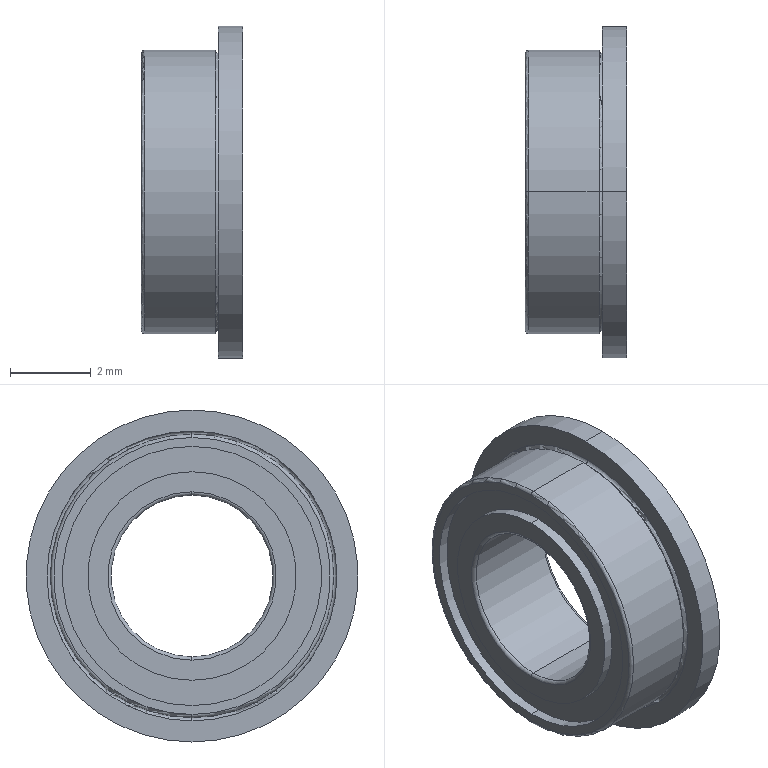Part | SolidWorks | features RefAxis 3, 3DProfileFeature 1, Revolution 1 | 1 solid | 31 faces | box 2.5 x 8.2 x 8.2 mm | volume 67.212 mm3 | cylinder 14 | torus 10 | plane 7 | commonest cylinder face diameters 5.15 x4 6.4 x4 4 x2 7 x2 8.2 x2
STEP:
#1=CARTESIAN_POINT('',(1.82,0.,3.5));
#2=VERTEX_POINT('',#1);
#3=CARTESIAN_POINT('',(1.9,0.,3.42));
#4=VERTEX_POINT('',#3);
#5=CARTESIAN_POINT('',(1.9,0.,3.5));
#6=DIRECTION('',(0.,-1.,0.));
#7=DIRECTION('',(0.,0.,-1.));
#8=AXIS2_PLACEMENT_3D('',#5,#6,#7);
#9=CIRCLE('',#8,0.08);
#10=EDGE_CURVE('',#2,#4,#9,.T.);
#11=ORIENTED_EDGE('',*,*,#10,.T.);
#12=CARTESIAN_POINT('',(1.9,0.,-3.42));
#13=VERTEX_POINT('',#12);
#14=CARTESIAN_POINT('',(1.9,0.,0.));
#15=DIRECTION('',(-1.,0.,0.));
#16=DIRECTION('',(0.,0.,1.));
#17=AXIS2_PLACEMENT_3D('',#14,#15,#16);
#18=CIRCLE('',#17,3.42);
#19=EDGE_CURVE('',#4,#13,#18,.T.);
#20=ORIENTED_EDGE('',*,*,#19,.T.);
#21=CARTESIAN_POINT('',(1.82,0.,-3.5));
#22=VERTEX_POINT('',#21);
#23=CARTESIAN_POINT('',(1.9,0.,-3.5));
#24=DIRECTION('',(0.,1.,0.));
#25=DIRECTION('',(0.,0.,1.));
#26=AXIS2_PLACEMENT_3D('',#23,#24,#25);
#27=CIRCLE('',#26,0.08);
#28=EDGE_CURVE('',#22,#13,#27,.T.);
#29=ORIENTED_EDGE('',*,*,#28,.F.);
#30=CARTESIAN_POINT('',(1.82,0.,0.));
#31=DIRECTION('',(-1.,0.,0.));
#32=DIRECTION('',(0.,0.,1.));
#33=AXIS2_PLACEMENT_3D('',#30,#31,#32);
#34=CIRCLE('',#33,3.5);
#35=EDGE_CURVE('',#2,#22,#34,.T.);
#36=ORIENTED_EDGE('',*,*,#35,.F.);
#37=EDGE_LOOP('',(#11,#20,#29,#36));
#38=FACE_OUTER_BOUND('',#37,.T.);
#39=CARTESIAN_POINT('',(1.9,0.,0.));
#40=DIRECTION('',(-1.,0.,0.));
#41=DIRECTION('',(0.,0.,1.));
#42=AXIS2_PLACEMENT_3D('',#39,#40,#41);
#43=TOROIDAL_SURFACE('',#42,3.5,0.08);
#44=ADVANCED_FACE('',(#38),#43,.F.);
#45=ORIENTED_EDGE('',*,*,#28,.T.);
#46=CARTESIAN_POINT('',(1.9,0.,0.));
#47=DIRECTION('',(-1.,0.,0.));
#48=DIRECTION('',(0.,0.,1.));
#49=AXIS2_PLACEMENT_3D('',#46,#47,#48);
#50=CIRCLE('',#49,3.42);
#51=EDGE_CURVE('',#13,#4,#50,.T.);
#52=ORIENTED_EDGE('',*,*,#51,.T.);
#53=ORIENTED_EDGE('',*,*,#10,.F.);
#54=CARTESIAN_POINT('',(1.82,0.,0.));
#55=DIRECTION('',(-1.,0.,0.));
#56=DIRECTION('',(0.,0.,1.));
#57=AXIS2_PLACEMENT_3D('',#54,#55,#56);
#58=CIRCLE('',#57,3.5);
#59=EDGE_CURVE('',#22,#2,#58,.T.);
#60=ORIENTED_EDGE('',*,*,#59,.F.);
#61=EDGE_LOOP('',(#45,#52,#53,#60));
#62=FACE_OUTER_BOUND('',#61,.T.);
#63=CARTESIAN_POINT('',(1.9,0.,0.));
#64=DIRECTION('',(-1.,0.,0.));
#65=DIRECTION('',(0.,0.,1.));
#66=AXIS2_PLACEMENT_3D('',#63,#64,#65);
#67=TOROIDAL_SURFACE('',#66,3.5,0.08);
#68=ADVANCED_FACE('',(#62),#67,.F.);
#69=ORIENTED_EDGE('',*,*,#35,.T.);
#70=CARTESIAN_POINT('',(0.08,0.,-3.5));
#71=VERTEX_POINT('',#70);
#72=CARTESIAN_POINT('',(7.,0.,-3.5));
#73=DIRECTION('',(-1.,0.,0.));
#74=VECTOR('',#73,1000.);
#75=LINE('',#72,#74);
#76=EDGE_CURVE('',#22,#71,#75,.T.);
#77=ORIENTED_EDGE('',*,*,#76,.T.);
#78=CARTESIAN_POINT('',(0.08,0.,3.5));
#79=VERTEX_POINT('',#78);
#80=CARTESIAN_POINT('',(0.08,0.,0.));
#81=DIRECTION('',(-1.,0.,0.));
#82=DIRECTION('',(0.,0.,1.));
#83=AXIS2_PLACEMENT_3D('',#80,#81,#82);
#84=CIRCLE('',#83,3.5);
#85=EDGE_CURVE('',#79,#71,#84,.T.);
#86=ORIENTED_EDGE('',*,*,#85,.F.);
#87=CARTESIAN_POINT('',(7.,0.,3.5));
#88=DIRECTION('',(-1.,0.,0.));
#89=VECTOR('',#88,1000.);
#90=LINE('',#87,#89);
#91=EDGE_CURVE('',#2,#79,#90,.T.);
#92=ORIENTED_EDGE('',*,*,#91,.F.);
#93=EDGE_LOOP('',(#69,#77,#86,#92));
#94=FACE_OUTER_BOUND('',#93,.T.);
#95=CARTESIAN_POINT('',(7.,0.,0.));
#96=DIRECTION('',(-1.,0.,0.));
#97=DIRECTION('',(0.,0.,1.));
#98=AXIS2_PLACEMENT_3D('',#95,#96,#97);
#99=CYLINDRICAL_SURFACE('',#98,3.5);
#100=ADVANCED_FACE('',(#94),#99,.T.);
#101=ORIENTED_EDGE('',*,*,#51,.F.);
#102=CARTESIAN_POINT('',(1.9,0.,-3.58));
#103=VERTEX_POINT('',#102);
#104=CARTESIAN_POINT('',(1.9,0.,-3.5));
#105=DIRECTION('',(0.,1.,0.));
#106=DIRECTION('',(0.,0.,1.));
#107=AXIS2_PLACEMENT_3D('',#104,#105,#106);
#108=CIRCLE('',#107,0.08);
#109=EDGE_CURVE('',#13,#103,#108,.T.);
#110=ORIENTED_EDGE('',*,*,#109,.T.);
#111=CARTESIAN_POINT('',(1.9,0.,3.58));
#112=VERTEX_POINT('',#111);
#113=CARTESIAN_POINT('',(1.9,0.,0.));
#114=DIRECTION('',(-1.,0.,0.));
#115=DIRECTION('',(0.,0.,1.));
#116=AXIS2_PLACEMENT_3D('',#113,#114,#115);
#117=CIRCLE('',#116,3.58);
#118=EDGE_CURVE('',#103,#112,#117,.T.);
#119=ORIENTED_EDGE('',*,*,#118,.T.);
#120=CARTESIAN_POINT('',(1.9,0.,3.5));
#121=DIRECTION('',(0.,-1.,0.));
#122=DIRECTION('',(0.,0.,-1.));
#123=AXIS2_PLACEMENT_3D('',#120,#121,#122);
#124=CIRCLE('',#123,0.08);
#125=EDGE_CURVE('',#4,#112,#124,.T.);
#126=ORIENTED_EDGE('',*,*,#125,.F.);
#127=EDGE_LOOP('',(#101,#110,#119,#126));
#128=FACE_OUTER_BOUND('',#127,.T.);
#129=CARTESIAN_POINT('',(1.9,0.,0.));
#130=DIRECTION('',(-1.,0.,0.));
#131=DIRECTION('',(0.,0.,1.));
#132=AXIS2_PLACEMENT_3D('',#129,#130,#131);
#133=TOROIDAL_SURFACE('',#132,3.5,0.08);
#134=ADVANCED_FACE('',(#128),#133,.F.);
#135=CARTESIAN_POINT('',(2.5,0.,4.1));
#136=VERTEX_POINT('',#135);
#137=CARTESIAN_POINT('',(2.5,0.,-4.1));
#138=VERTEX_POINT('',#137);
#139=CARTESIAN_POINT('',(2.5,0.,0.));
#140=DIRECTION('',(-1.,0.,0.));
#141=DIRECTION('',(0.,0.,1.));
#142=AXIS2_PLACEMENT_3D('',#139,#140,#141);
#143=CIRCLE('',#142,4.1);
#144=EDGE_CURVE('',#136,#138,#143,.T.);
#145=ORIENTED_EDGE('',*,*,#144,.T.);
#146=CARTESIAN_POINT('',(1.9,0.,-4.1));
#147=VERTEX_POINT('',#146);
#148=CARTESIAN_POINT('',(7.,0.,-4.1));
#149=DIRECTION('',(-1.,0.,0.));
#150=VECTOR('',#149,1000.);
#151=LINE('',#148,#150);
#152=EDGE_CURVE('',#138,#147,#151,.T.);
#153=ORIENTED_EDGE('',*,*,#152,.T.);
#154=CARTESIAN_POINT('',(1.9,0.,4.1));
#155=VERTEX_POINT('',#154);
#156=CARTESIAN_POINT('',(1.9,0.,0.));
#157=DIRECTION('',(-1.,0.,0.));
#158=DIRECTION('',(0.,0.,1.));
#159=AXIS2_PLACEMENT_3D('',#156,#157,#158);
#160=CIRCLE('',#159,4.1);
#161=EDGE_CURVE('',#155,#147,#160,.T.);
#162=ORIENTED_EDGE('',*,*,#161,.F.);
#163=CARTESIAN_POINT('',(7.,0.,4.1));
#164=DIRECTION('',(-1.,0.,0.));
#165=VECTOR('',#164,1000.);
#166=LINE('',#163,#165);
#167=EDGE_CURVE('',#136,#155,#166,.T.);
#168=ORIENTED_EDGE('',*,*,#167,.F.);
#169=EDGE_LOOP('',(#145,#153,#162,#168));
#170=FACE_OUTER_BOUND('',#169,.T.);
#171=CARTESIAN_POINT('',(7.,0.,0.));
#172=DIRECTION('',(-1.,0.,0.));
#173=DIRECTION('',(0.,0.,1.));
#174=AXIS2_PLACEMENT_3D('',#171,#172,#173);
#175=CYLINDRICAL_SURFACE('',#174,4.1);
#176=ADVANCED_FACE('',(#170),#175,.T.);
#177=CARTESIAN_POINT('',(2.5,0.,-3.2));
#178=VERTEX_POINT('',#177);
#179=CARTESIAN_POINT('',(2.5,0.,3.2));
#180=VERTEX_POINT('',#179);
#181=CARTESIAN_POINT('',(2.5,0.,0.));
#182=DIRECTION('',(-1.,0.,0.));
#183=DIRECTION('',(0.,0.,1.));
#184=AXIS2_PLACEMENT_3D('',#181,#182,#183);
#185=CIRCLE('',#184,3.2);
#186=EDGE_CURVE('',#178,#180,#185,.T.);
#187=ORIENTED_EDGE('',*,*,#186,.F.);
#188=CARTESIAN_POINT('',(2.245,0.,-3.2));
#189=VERTEX_POINT('',#188);
#190=CARTESIAN_POINT('',(7.,0.,-3.2));
#191=DIRECTION('',(-1.,0.,0.));
#192=VECTOR('',#191,1000.);
#193=LINE('',#190,#192);
#194=EDGE_CURVE('',#178,#189,#193,.T.);
#195=ORIENTED_EDGE('',*,*,#194,.T.);
#196=CARTESIAN_POINT('',(2.245,0.,3.2));
#197=VERTEX_POINT('',#196);
#198=CARTESIAN_POINT('',(2.245,0.,0.));
#199=DIRECTION('',(-1.,0.,0.));
#200=DIRECTION('',(0.,0.,1.));
#201=AXIS2_PLACEMENT_3D('',#198,#199,#200);
#202=CIRCLE('',#201,3.2);
#203=EDGE_CURVE('',#189,#197,#202,.T.);
#204=ORIENTED_EDGE('',*,*,#203,.T.);
#205=CARTESIAN_POINT('',(7.,0.,3.2));
#206=DIRECTION('',(-1.,0.,0.));
#207=VECTOR('',#206,1000.);
#208=LINE('',#205,#207);
#209=EDGE_CURVE('',#180,#197,#208,.T.);
#210=ORIENTED_EDGE('',*,*,#209,.F.);
#211=EDGE_LOOP('',(#187,#195,#204,#210));
#212=FACE_OUTER_BOUND('',#211,.T.);
#213=CARTESIAN_POINT('',(7.,0.,0.));
#214=DIRECTION('',(-1.,0.,0.));
#215=DIRECTION('',(0.,0.,1.));
#216=AXIS2_PLACEMENT_3D('',#213,#214,#215);
#217=CYLINDRICAL_SURFACE('',#216,3.2);
#218=ADVANCED_FACE('',(#212),#217,.F.);
#219=CARTESIAN_POINT('',(2.5,0.,2.575));
#220=VERTEX_POINT('',#219);
#221=CARTESIAN_POINT('',(2.5,0.,-2.575));
#222=VERTEX_POINT('',#221);
#223=CARTESIAN_POINT('',(2.5,0.,0.));
#224=DIRECTION('',(-1.,0.,0.));
#225=DIRECTION('',(0.,0.,1.));
#226=AXIS2_PLACEMENT_3D('',#223,#224,#225);
#227=CIRCLE('',#226,2.575);
#228=EDGE_CURVE('',#220,#222,#227,.T.);
#229=ORIENTED_EDGE('',*,*,#228,.T.);
#230=CARTESIAN_POINT('',(2.245,0.,-2.575));
#231=VERTEX_POINT('',#230);
#232=CARTESIAN_POINT('',(7.,0.,-2.575));
#233=DIRECTION('',(-1.,0.,0.));
#234=VECTOR('',#233,1000.);
#235=LINE('',#232,#234);
#236=EDGE_CURVE('',#222,#231,#235,.T.);
#237=ORIENTED_EDGE('',*,*,#236,.T.);
#238=CARTESIAN_POINT('',(2.245,0.,2.575));
#239=VERTEX_POINT('',#238);
#240=CARTESIAN_POINT('',(2.245,0.,0.));
#241=DIRECTION('',(-1.,0.,0.));
#242=DIRECTION('',(0.,0.,1.));
#243=AXIS2_PLACEMENT_3D('',#240,#241,#242);
#244=CIRCLE('',#243,2.575);
#245=EDGE_CURVE('',#239,#231,#244,.T.);
#246=ORIENTED_EDGE('',*,*,#245,.F.);
#247=CARTESIAN_POINT('',(7.,0.,2.575));
#248=DIRECTION('',(-1.,0.,0.));
#249=VECTOR('',#248,1000.);
#250=LINE('',#247,#249);
#251=EDGE_CURVE('',#220,#239,#250,.T.);
#252=ORIENTED_EDGE('',*,*,#251,.F.);
#253=EDGE_LOOP('',(#229,#237,#246,#252));
#254=FACE_OUTER_BOUND('',#253,.T.);
#255=CARTESIAN_POINT('',(7.,0.,0.));
#256=DIRECTION('',(-1.,0.,0.));
#257=DIRECTION('',(0.,0.,1.));
#258=AXIS2_PLACEMENT_3D('',#255,#256,#257);
#259=CYLINDRICAL_SURFACE('',#258,2.575);
#260=ADVANCED_FACE('',(#254),#259,.T.);
#261=CARTESIAN_POINT('',(2.42,0.,2.));
#262=VERTEX_POINT('',#261);
#263=CARTESIAN_POINT('',(2.42,0.,-2.));
#264=VERTEX_POINT('',#263);
#265=CARTESIAN_POINT('',(2.42,0.,0.));
#266=DIRECTION('',(-1.,0.,0.));
#267=DIRECTION('',(0.,0.,1.));
#268=AXIS2_PLACEMENT_3D('',#265,#266,#267);
#269=CIRCLE('',#268,2.);
#270=EDGE_CURVE('',#262,#264,#269,.T.);
#271=ORIENTED_EDGE('',*,*,#270,.T.);
#272=CARTESIAN_POINT('',(2.5,0.,-2.08));
#273=VERTEX_POINT('',#272);
#274=CARTESIAN_POINT('',(2.42,0.,-2.08));
#275=DIRECTION('',(0.,1.,0.));
#276=DIRECTION('',(0.,0.,1.));
#277=AXIS2_PLACEMENT_3D('',#274,#275,#276);
#278=CIRCLE('',#277,0.08);
#279=EDGE_CURVE('',#264,#273,#278,.T.);
#280=ORIENTED_EDGE('',*,*,#279,.T.);
#281=CARTESIAN_POINT('',(2.5,0.,2.08));
#282=VERTEX_POINT('',#281);
#283=CARTESIAN_POINT('',(2.5,0.,0.));
#284=DIRECTION('',(-1.,0.,0.));
#285=DIRECTION('',(0.,0.,1.));
#286=AXIS2_PLACEMENT_3D('',#283,#284,#285);
#287=CIRCLE('',#286,2.08);
#288=EDGE_CURVE('',#282,#273,#287,.T.);
#289=ORIENTED_EDGE('',*,*,#288,.F.);
#290=CARTESIAN_POINT('',(2.42,0.,2.08));
#291=DIRECTION('',(0.,-1.,0.));
#292=DIRECTION('',(0.,0.,-1.));
#293=AXIS2_PLACEMENT_3D('',#290,#291,#292);
#294=CIRCLE('',#293,0.08);
#295=EDGE_CURVE('',#262,#282,#294,.T.);
#296=ORIENTED_EDGE('',*,*,#295,.F.);
#297=EDGE_LOOP('',(#271,#280,#289,#296));
#298=FACE_OUTER_BOUND('',#297,.T.);
#299=CARTESIAN_POINT('',(2.42,0.,0.));
#300=DIRECTION('',(-1.,0.,0.));
#301=DIRECTION('',(0.,0.,1.));
#302=AXIS2_PLACEMENT_3D('',#299,#300,#301);
#303=TOROIDAL_SURFACE('',#302,2.08,0.08);
#304=ADVANCED_FACE('',(#298),#303,.T.);
#305=CARTESIAN_POINT('',(2.42,0.,0.));
#306=DIRECTION('',(-1.,0.,0.));
#307=DIRECTION('',(0.,0.,1.));
#308=AXIS2_PLACEMENT_3D('',#305,#306,#307);
#309=CIRCLE('',#308,2.);
#310=EDGE_CURVE('',#264,#262,#309,.T.);
#311=ORIENTED_EDGE('',*,*,#310,.F.);
#312=CARTESIAN_POINT('',(0.08,0.,-2.));
#313=VERTEX_POINT('',#312);
#314=CARTESIAN_POINT('',(7.,0.,-2.));
#315=DIRECTION('',(-1.,0.,0.));
#316=VECTOR('',#315,1000.);
#317=LINE('',#314,#316);
#318=EDGE_CURVE('',#264,#313,#317,.T.);
#319=ORIENTED_EDGE('',*,*,#318,.T.);
#320=CARTESIAN_POINT('',(0.08,0.,2.));
#321=VERTEX_POINT('',#320);
#322=CARTESIAN_POINT('',(0.08,0.,0.));
#323=DIRECTION('',(-1.,0.,0.));
#324=DIRECTION('',(0.,0.,1.));
#325=AXIS2_PLACEMENT_3D('',#322,#323,#324);
#326=CIRCLE('',#325,2.);
#327=EDGE_CURVE('',#313,#321,#326,.T.);
#328=ORIENTED_EDGE('',*,*,#327,.T.);
#329=CARTESIAN_POINT('',(7.,0.,2.));
#330=DIRECTION('',(-1.,0.,0.));
#331=VECTOR('',#330,1000.);
#332=LINE('',#329,#331);
#333=EDGE_CURVE('',#262,#321,#332,.T.);
#334=ORIENTED_EDGE('',*,*,#333,.F.);
#335=EDGE_LOOP('',(#311,#319,#328,#334));
#336=FACE_OUTER_BOUND('',#335,.T.);
#337=CARTESIAN_POINT('',(7.,0.,0.));
#338=DIRECTION('',(-1.,0.,0.));
#339=DIRECTION('',(0.,0.,1.));
#340=AXIS2_PLACEMENT_3D('',#337,#338,#339);
#341=CYLINDRICAL_SURFACE('',#340,2.);
#342=ADVANCED_FACE('',(#336),#341,.F.);
#343=CARTESIAN_POINT('',(0.,0.,2.08));
#344=VERTEX_POINT('',#343);
#345=CARTESIAN_POINT('',(0.,0.,-2.08));
#346=VERTEX_POINT('',#345);
#347=CARTESIAN_POINT('',(0.,0.,0.));
#348=DIRECTION('',(-1.,0.,0.));
#349=DIRECTION('',(0.,0.,1.));
#350=AXIS2_PLACEMENT_3D('',#347,#348,#349);
#351=CIRCLE('',#350,2.08);
#352=EDGE_CURVE('',#344,#346,#351,.T.);
#353=ORIENTED_EDGE('',*,*,#352,.T.);
#354=CARTESIAN_POINT('',(0.08,0.,-2.08));
#355=DIRECTION('',(0.,1.,0.));
#356=DIRECTION('',(0.,0.,1.));
#357=AXIS2_PLACEMENT_3D('',#354,#355,#356);
#358=CIRCLE('',#357,0.08);
#359=EDGE_CURVE('',#346,#313,#358,.T.);
#360=ORIENTED_EDGE('',*,*,#359,.T.);
#361=CARTESIAN_POINT('',(0.08,0.,0.));
#362=DIRECTION('',(-1.,0.,0.));
#363=DIRECTION('',(0.,0.,1.));
#364=AXIS2_PLACEMENT_3D('',#361,#362,#363);
#365=CIRCLE('',#364,2.);
#366=EDGE_CURVE('',#321,#313,#365,.T.);
#367=ORIENTED_EDGE('',*,*,#366,.F.);
#368=CARTESIAN_POINT('',(0.08,0.,2.08));
#369=DIRECTION('',(0.,-1.,0.));
#370=DIRECTION('',(0.,0.,-1.));
#371=AXIS2_PLACEMENT_3D('',#368,#369,#370);
#372=CIRCLE('',#371,0.08);
#373=EDGE_CURVE('',#344,#321,#372,.T.);
#374=ORIENTED_EDGE('',*,*,#373,.F.);
#375=EDGE_LOOP('',(#353,#360,#367,#374));
#376=FACE_OUTER_BOUND('',#375,.T.);
#377=CARTESIAN_POINT('',(0.08,0.,0.));
#378=DIRECTION('',(-1.,0.,0.));
#379=DIRECTION('',(0.,0.,1.));
#380=AXIS2_PLACEMENT_3D('',#377,#378,#379);
#381=TOROIDAL_SURFACE('',#380,2.08,0.08);
#382=ADVANCED_FACE('',(#376),#381,.T.);
#383=CARTESIAN_POINT('',(0.255,0.,2.575));
#384=VERTEX_POINT('',#383);
#385=CARTESIAN_POINT('',(0.255,0.,-2.575));
#386=VERTEX_POINT('',#385);
#387=CARTESIAN_POINT('',(0.255,0.,0.));
#388=DIRECTION('',(-1.,0.,0.));
#389=DIRECTION('',(0.,0.,1.));
#390=AXIS2_PLACEMENT_3D('',#387,#388,#389);
#391=CIRCLE('',#390,2.575);
#392=EDGE_CURVE('',#384,#386,#391,.T.);
#393=ORIENTED_EDGE('',*,*,#392,.T.);
#394=CARTESIAN_POINT('',(0.,0.,-2.575));
#395=VERTEX_POINT('',#394);
#396=CARTESIAN_POINT('',(7.,0.,-2.575));
#397=DIRECTION('',(-1.,0.,0.));
#398=VECTOR('',#397,1000.);
#399=LINE('',#396,#398);
#400=EDGE_CURVE('',#386,#395,#399,.T.);
#401=ORIENTED_EDGE('',*,*,#400,.T.);
#402=CARTESIAN_POINT('',(0.,0.,2.575));
#403=VERTEX_POINT('',#402);
#404=CARTESIAN_POINT('',(0.,0.,0.));
#405=DIRECTION('',(-1.,0.,0.));
#406=DIRECTION('',(0.,0.,1.));
#407=AXIS2_PLACEMENT_3D('',#404,#405,#406);
#408=CIRCLE('',#407,2.575);
#409=EDGE_CURVE('',#403,#395,#408,.T.);
#410=ORIENTED_EDGE('',*,*,#409,.F.);
#411=CARTESIAN_POINT('',(7.,0.,2.575));
#412=DIRECTION('',(-1.,0.,0.));
#413=VECTOR('',#412,1000.);
#414=LINE('',#411,#413);
#415=EDGE_CURVE('',#384,#403,#414,.T.);
#416=ORIENTED_EDGE('',*,*,#415,.F.);
#417=EDGE_LOOP('',(#393,#401,#410,#416));
#418=FACE_OUTER_BOUND('',#417,.T.);
#419=CARTESIAN_POINT('',(7.,0.,0.));
#420=DIRECTION('',(-1.,0.,0.));
#421=DIRECTION('',(0.,0.,1.));
#422=AXIS2_PLACEMENT_3D('',#419,#420,#421);
#423=CYLINDRICAL_SURFACE('',#422,2.575);
#424=ADVANCED_FACE('',(#418),#423,.T.);
#425=CARTESIAN_POINT('',(0.255,0.,-3.2));
#426=VERTEX_POINT('',#425);
#427=CARTESIAN_POINT('',(0.255,0.,3.2));
#428=VERTEX_POINT('',#427);
#429=CARTESIAN_POINT('',(0.255,0.,0.));
#430=DIRECTION('',(-1.,0.,0.));
#431=DIRECTION('',(0.,0.,1.));
#432=AXIS2_PLACEMENT_3D('',#429,#430,#431);
#433=CIRCLE('',#432,3.2);
#434=EDGE_CURVE('',#426,#428,#433,.T.);
#435=ORIENTED_EDGE('',*,*,#434,.F.);
#436=CARTESIAN_POINT('',(0.,0.,-3.2));
#437=VERTEX_POINT('',#436);
#438=CARTESIAN_POINT('',(7.,0.,-3.2));
#439=DIRECTION('',(-1.,0.,0.));
#440=VECTOR('',#439,1000.);
#441=LINE('',#438,#440);
#442=EDGE_CURVE('',#426,#437,#441,.T.);
#443=ORIENTED_EDGE('',*,*,#442,.T.);
#444=CARTESIAN_POINT('',(0.,0.,3.2));
#445=VERTEX_POINT('',#444);
#446=CARTESIAN_POINT('',(0.,0.,0.));
#447=DIRECTION('',(-1.,0.,0.));
#448=DIRECTION('',(0.,0.,1.));
#449=AXIS2_PLACEMENT_3D('',#446,#447,#448);
#450=CIRCLE('',#449,3.2);
#451=EDGE_CURVE('',#437,#445,#450,.T.);
#452=ORIENTED_EDGE('',*,*,#451,.T.);
#453=CARTESIAN_POINT('',(7.,0.,3.2));
#454=DIRECTION('',(-1.,0.,0.));
#455=VECTOR('',#454,1000.);
#456=LINE('',#453,#455);
#457=EDGE_CURVE('',#428,#445,#456,.T.);
#458=ORIENTED_EDGE('',*,*,#457,.F.);
#459=EDGE_LOOP('',(#435,#443,#452,#458));
#460=FACE_OUTER_BOUND('',#459,.T.);
#461=CARTESIAN_POINT('',(7.,0.,0.));
#462=DIRECTION('',(-1.,0.,0.));
#463=DIRECTION('',(0.,0.,1.));
#464=AXIS2_PLACEMENT_3D('',#461,#462,#463);
#465=CYLINDRICAL_SURFACE('',#464,3.2);
#466=ADVANCED_FACE('',(#460),#465,.F.);
#467=ORIENTED_EDGE('',*,*,#85,.T.);
#468=CARTESIAN_POINT('',(0.,0.,-3.42));
#469=VERTEX_POINT('',#468);
#470=CARTESIAN_POINT('',(0.08,0.,-3.42));
#471=DIRECTION('',(0.,1.,0.));
#472=DIRECTION('',(0.,0.,1.));
#473=AXIS2_PLACEMENT_3D('',#470,#471,#472);
#474=CIRCLE('',#473,0.08);
#475=EDGE_CURVE('',#71,#469,#474,.T.);
#476=ORIENTED_EDGE('',*,*,#475,.T.);
#477=CARTESIAN_POINT('',(0.,0.,3.42));
#478=VERTEX_POINT('',#477);
#479=CARTESIAN_POINT('',(0.,0.,0.));
#480=DIRECTION('',(-1.,0.,0.));
#481=DIRECTION('',(0.,0.,1.));
#482=AXIS2_PLACEMENT_3D('',#479,#480,#481);
#483=CIRCLE('',#482,3.42);
#484=EDGE_CURVE('',#478,#469,#483,.T.);
#485=ORIENTED_EDGE('',*,*,#484,.F.);
#486=CARTESIAN_POINT('',(0.08,0.,3.42));
#487=DIRECTION('',(0.,-1.,0.));
#488=DIRECTION('',(0.,0.,-1.));
#489=AXIS2_PLACEMENT_3D('',#486,#487,#488);
#490=CIRCLE('',#489,0.08);
#491=EDGE_CURVE('',#79,#478,#490,.T.);
#492=ORIENTED_EDGE('',*,*,#491,.F.);
#493=EDGE_LOOP('',(#467,#476,#485,#492));
#494=FACE_OUTER_BOUND('',#493,.T.);
#495=CARTESIAN_POINT('',(0.08,0.,0.));
#496=DIRECTION('',(-1.,0.,0.));
#497=DIRECTION('',(0.,0.,1.));
#498=AXIS2_PLACEMENT_3D('',#495,#496,#497);
#499=TOROIDAL_SURFACE('',#498,3.42,0.08);
#500=ADVANCED_FACE('',(#494),#499,.T.);
#501=ORIENTED_EDGE('',*,*,#475,.F.);
#502=CARTESIAN_POINT('',(0.08,0.,0.));
#503=DIRECTION('',(-1.,0.,0.));
#504=DIRECTION('',(0.,0.,1.));
#505=AXIS2_PLACEMENT_3D('',#502,#503,#504);
#506=CIRCLE('',#505,3.5);
#507=EDGE_CURVE('',#71,#79,#506,.T.);
#508=ORIENTED_EDGE('',*,*,#507,.T.);
#509=ORIENTED_EDGE('',*,*,#491,.T.);
#510=CARTESIAN_POINT('',(0.,0.,0.));
#511=DIRECTION('',(-1.,0.,0.));
#512=DIRECTION('',(0.,0.,1.));
#513=AXIS2_PLACEMENT_3D('',#510,#511,#512);
#514=CIRCLE('',#513,3.42);
#515=EDGE_CURVE('',#469,#478,#514,.T.);
#516=ORIENTED_EDGE('',*,*,#515,.F.);
#517=EDGE_LOOP('',(#501,#508,#509,#516));
#518=FACE_OUTER_BOUND('',#517,.T.);
#519=CARTESIAN_POINT('',(0.08,0.,0.));
#520=DIRECTION('',(-1.,0.,0.));
#521=DIRECTION('',(0.,0.,1.));
#522=AXIS2_PLACEMENT_3D('',#519,#520,#521);
#523=TOROIDAL_SURFACE('',#522,3.42,0.08);
#524=ADVANCED_FACE('',(#518),#523,.T.);
#525=CARTESIAN_POINT('',(0.,0.,0.));
#526=DIRECTION('',(-1.,0.,0.));
#527=DIRECTION('',(0.,0.,1.));
#528=AXIS2_PLACEMENT_3D('',#525,#526,#527);
#529=CIRCLE('',#528,3.2);
#530=EDGE_CURVE('',#445,#437,#529,.T.);
#531=ORIENTED_EDGE('',*,*,#530,.F.);
#532=ORIENTED_EDGE('',*,*,#451,.F.);
#533=EDGE_LOOP('',(#531,#532));
#534=FACE_BOUND('',#533,.T.);
#535=ORIENTED_EDGE('',*,*,#484,.T.);
#536=ORIENTED_EDGE('',*,*,#515,.T.);
#537=EDGE_LOOP('',(#535,#536));
#538=FACE_OUTER_BOUND('',#537,.T.);
#539=CARTESIAN_POINT('',(0.,3.42,0.));
#540=DIRECTION('',(1.,0.,0.));
#541=DIRECTION('',(0.,0.,-1.));
#542=AXIS2_PLACEMENT_3D('',#539,#540,#541);
#543=PLANE('',#542);
#544=ADVANCED_FACE('',(#534,#538),#543,.F.);
#545=ORIENTED_EDGE('',*,*,#442,.F.);
#546=CARTESIAN_POINT('',(0.255,0.,0.));
#547=DIRECTION('',(-1.,0.,0.));
#548=DIRECTION('',(0.,0.,1.));
#549=AXIS2_PLACEMENT_3D('',#546,#547,#548);
#550=CIRCLE('',#549,3.2);
#551=EDGE_CURVE('',#428,#426,#550,.T.);
#552=ORIENTED_EDGE('',*,*,#551,.F.);
#553=ORIENTED_EDGE('',*,*,#457,.T.);
#554=ORIENTED_EDGE('',*,*,#530,.T.);
#555=EDGE_LOOP('',(#545,#552,#553,#554));
#556=FACE_OUTER_BOUND('',#555,.T.);
#557=CARTESIAN_POINT('',(7.,0.,0.));
#558=DIRECTION('',(-1.,0.,0.));
#559=DIRECTION('',(0.,0.,1.));
#560=AXIS2_PLACEMENT_3D('',#557,#558,#559);
#561=CYLINDRICAL_SURFACE('',#560,3.2);
#562=ADVANCED_FACE('',(#556),#561,.F.);
#563=ORIENTED_EDGE('',*,*,#392,.F.);
#564=CARTESIAN_POINT('',(0.255,0.,0.));
#565=DIRECTION('',(-1.,0.,0.));
#566=DIRECTION('',(0.,0.,1.));
#567=AXIS2_PLACEMENT_3D('',#564,#565,#566);
#568=CIRCLE('',#567,2.575);
#569=EDGE_CURVE('',#386,#384,#568,.T.);
#570=ORIENTED_EDGE('',*,*,#569,.F.);
#571=EDGE_LOOP('',(#563,#570));
#572=FACE_BOUND('',#571,.T.);
#573=ORIENTED_EDGE('',*,*,#551,.T.);
#574=ORIENTED_EDGE('',*,*,#434,.T.);
#575=EDGE_LOOP('',(#573,#574));
#576=FACE_OUTER_BOUND('',#575,.T.);
#577=CARTESIAN_POINT('',(0.255,3.2,0.));
#578=DIRECTION('',(1.,0.,0.));
#579=DIRECTION('',(0.,0.,-1.));
#580=AXIS2_PLACEMENT_3D('',#577,#578,#579);
#581=PLANE('',#580);
#582=ADVANCED_FACE('',(#572,#576),#581,.F.);
#583=ORIENTED_EDGE('',*,*,#400,.F.);
#584=ORIENTED_EDGE('',*,*,#569,.T.);
#585=ORIENTED_EDGE('',*,*,#415,.T.);
#586=CARTESIAN_POINT('',(0.,0.,0.));
#587=DIRECTION('',(-1.,0.,0.));
#588=DIRECTION('',(0.,0.,1.));
#589=AXIS2_PLACEMENT_3D('',#586,#587,#588);
#590=CIRCLE('',#589,2.575);
#591=EDGE_CURVE('',#395,#403,#590,.T.);
#592=ORIENTED_EDGE('',*,*,#591,.F.);
#593=EDGE_LOOP('',(#583,#584,#585,#592));
#594=FACE_OUTER_BOUND('',#593,.T.);
#595=CARTESIAN_POINT('',(7.,0.,0.));
#596=DIRECTION('',(-1.,0.,0.));
#597=DIRECTION('',(0.,0.,1.));
#598=AXIS2_PLACEMENT_3D('',#595,#596,#597);
#599=CYLINDRICAL_SURFACE('',#598,2.575);
#600=ADVANCED_FACE('',(#594),#599,.T.);
#601=ORIENTED_EDGE('',*,*,#352,.F.);
#602=CARTESIAN_POINT('',(0.,0.,0.));
#603=DIRECTION('',(-1.,0.,0.));
#604=DIRECTION('',(0.,0.,1.));
#605=AXIS2_PLACEMENT_3D('',#602,#603,#604);
#606=CIRCLE('',#605,2.08);
#607=EDGE_CURVE('',#346,#344,#606,.T.);
#608=ORIENTED_EDGE('',*,*,#607,.F.);
#609=EDGE_LOOP('',(#601,#608));
#610=FACE_BOUND('',#609,.T.);
#611=ORIENTED_EDGE('',*,*,#409,.T.);
#612=ORIENTED_EDGE('',*,*,#591,.T.);
#613=EDGE_LOOP('',(#611,#612));
#614=FACE_OUTER_BOUND('',#613,.T.);
#615=CARTESIAN_POINT('',(0.,2.575,0.));
#616=DIRECTION('',(1.,0.,0.));
#617=DIRECTION('',(0.,0.,-1.));
#618=AXIS2_PLACEMENT_3D('',#615,#616,#617);
#619=PLANE('',#618);
#620=ADVANCED_FACE('',(#610,#614),#619,.F.);
#621=ORIENTED_EDGE('',*,*,#359,.F.);
#622=ORIENTED_EDGE('',*,*,#607,.T.);
#623=ORIENTED_EDGE('',*,*,#373,.T.);
#624=ORIENTED_EDGE('',*,*,#327,.F.);
#625=EDGE_LOOP('',(#621,#622,#623,#624));
#626=FACE_OUTER_BOUND('',#625,.T.);
#627=CARTESIAN_POINT('',(0.08,0.,0.));
#628=DIRECTION('',(-1.,0.,0.));
#629=DIRECTION('',(0.,0.,1.));
#630=AXIS2_PLACEMENT_3D('',#627,#628,#629);
#631=TOROIDAL_SURFACE('',#630,2.08,0.08);
#632=ADVANCED_FACE('',(#626),#631,.T.);
#633=ORIENTED_EDGE('',*,*,#318,.F.);
#634=ORIENTED_EDGE('',*,*,#270,.F.);
#635=ORIENTED_EDGE('',*,*,#333,.T.);
#636=ORIENTED_EDGE('',*,*,#366,.T.);
#637=EDGE_LOOP('',(#633,#634,#635,#636));
#638=FACE_OUTER_BOUND('',#637,.T.);
#639=CARTESIAN_POINT('',(7.,0.,0.));
#640=DIRECTION('',(-1.,0.,0.));
#641=DIRECTION('',(0.,0.,1.));
#642=AXIS2_PLACEMENT_3D('',#639,#640,#641);
#643=CYLINDRICAL_SURFACE('',#642,2.);
#644=ADVANCED_FACE('',(#638),#643,.F.);
#645=ORIENTED_EDGE('',*,*,#279,.F.);
#646=ORIENTED_EDGE('',*,*,#310,.T.);
#647=ORIENTED_EDGE('',*,*,#295,.T.);
#648=CARTESIAN_POINT('',(2.5,0.,0.));
#649=DIRECTION('',(-1.,0.,0.));
#650=DIRECTION('',(0.,0.,1.));
#651=AXIS2_PLACEMENT_3D('',#648,#649,#650);
#652=CIRCLE('',#651,2.08);
#653=EDGE_CURVE('',#273,#282,#652,.T.);
#654=ORIENTED_EDGE('',*,*,#653,.F.);
#655=EDGE_LOOP('',(#645,#646,#647,#654));
#656=FACE_OUTER_BOUND('',#655,.T.);
#657=CARTESIAN_POINT('',(2.42,0.,0.));
#658=DIRECTION('',(-1.,0.,0.));
#659=DIRECTION('',(0.,0.,1.));
#660=AXIS2_PLACEMENT_3D('',#657,#658,#659);
#661=TOROIDAL_SURFACE('',#660,2.08,0.08);
#662=ADVANCED_FACE('',(#656),#661,.T.);
#663=ORIENTED_EDGE('',*,*,#228,.F.);
#664=CARTESIAN_POINT('',(2.5,0.,0.));
#665=DIRECTION('',(-1.,0.,0.));
#666=DIRECTION('',(0.,0.,1.));
#667=AXIS2_PLACEMENT_3D('',#664,#665,#666);
#668=CIRCLE('',#667,2.575);
#669=EDGE_CURVE('',#222,#220,#668,.T.);
#670=ORIENTED_EDGE('',*,*,#669,.F.);
#671=EDGE_LOOP('',(#663,#670));
#672=FACE_OUTER_BOUND('',#671,.T.);
#673=ORIENTED_EDGE('',*,*,#288,.T.);
#674=ORIENTED_EDGE('',*,*,#653,.T.);
#675=EDGE_LOOP('',(#673,#674));
#676=FACE_BOUND('',#675,.T.);
#677=CARTESIAN_POINT('',(2.5,2.08,0.));
#678=DIRECTION('',(-1.,0.,0.));
#679=DIRECTION('',(0.,0.,1.));
#680=AXIS2_PLACEMENT_3D('',#677,#678,#679);
#681=PLANE('',#680);
#682=ADVANCED_FACE('',(#672,#676),#681,.F.);
#683=ORIENTED_EDGE('',*,*,#236,.F.);
#684=ORIENTED_EDGE('',*,*,#669,.T.);
#685=ORIENTED_EDGE('',*,*,#251,.T.);
#686=CARTESIAN_POINT('',(2.245,0.,0.));
#687=DIRECTION('',(-1.,0.,0.));
#688=DIRECTION('',(0.,0.,1.));
#689=AXIS2_PLACEMENT_3D('',#686,#687,#688);
#690=CIRCLE('',#689,2.575);
#691=EDGE_CURVE('',#231,#239,#690,.T.);
#692=ORIENTED_EDGE('',*,*,#691,.F.);
#693=EDGE_LOOP('',(#683,#684,#685,#692));
#694=FACE_OUTER_BOUND('',#693,.T.);
#695=CARTESIAN_POINT('',(7.,0.,0.));
#696=DIRECTION('',(-1.,0.,0.));
#697=DIRECTION('',(0.,0.,1.));
#698=AXIS2_PLACEMENT_3D('',#695,#696,#697);
#699=CYLINDRICAL_SURFACE('',#698,2.575);
#700=ADVANCED_FACE('',(#694),#699,.T.);
#701=CARTESIAN_POINT('',(2.245,0.,0.));
#702=DIRECTION('',(-1.,0.,0.));
#703=DIRECTION('',(0.,0.,1.));
#704=AXIS2_PLACEMENT_3D('',#701,#702,#703);
#705=CIRCLE('',#704,3.2);
#706=EDGE_CURVE('',#197,#189,#705,.T.);
#707=ORIENTED_EDGE('',*,*,#706,.F.);
#708=ORIENTED_EDGE('',*,*,#203,.F.);
#709=EDGE_LOOP('',(#707,#708));
#710=FACE_OUTER_BOUND('',#709,.T.);
#711=ORIENTED_EDGE('',*,*,#245,.T.);
#712=ORIENTED_EDGE('',*,*,#691,.T.);
#713=EDGE_LOOP('',(#711,#712));
#714=FACE_BOUND('',#713,.T.);
#715=CARTESIAN_POINT('',(2.245,2.575,0.));
#716=DIRECTION('',(-1.,0.,0.));
#717=DIRECTION('',(0.,0.,1.));
#718=AXIS2_PLACEMENT_3D('',#715,#716,#717);
#719=PLANE('',#718);
#720=ADVANCED_FACE('',(#710,#714),#719,.F.);
#721=ORIENTED_EDGE('',*,*,#194,.F.);
#722=CARTESIAN_POINT('',(2.5,0.,0.));
#723=DIRECTION('',(-1.,0.,0.));
#724=DIRECTION('',(0.,0.,1.));
#725=AXIS2_PLACEMENT_3D('',#722,#723,#724);
#726=CIRCLE('',#725,3.2);
#727=EDGE_CURVE('',#180,#178,#726,.T.);
#728=ORIENTED_EDGE('',*,*,#727,.F.);
#729=ORIENTED_EDGE('',*,*,#209,.T.);
#730=ORIENTED_EDGE('',*,*,#706,.T.);
#731=EDGE_LOOP('',(#721,#728,#729,#730));
#732=FACE_OUTER_BOUND('',#731,.T.);
#733=CARTESIAN_POINT('',(7.,0.,0.));
#734=DIRECTION('',(-1.,0.,0.));
#735=DIRECTION('',(0.,0.,1.));
#736=AXIS2_PLACEMENT_3D('',#733,#734,#735);
#737=CYLINDRICAL_SURFACE('',#736,3.2);
#738=ADVANCED_FACE('',(#732),#737,.F.);
#739=ORIENTED_EDGE('',*,*,#144,.F.);
#740=CARTESIAN_POINT('',(2.5,0.,0.));
#741=DIRECTION('',(-1.,0.,0.));
#742=DIRECTION('',(0.,0.,1.));
#743=AXIS2_PLACEMENT_3D('',#740,#741,#742);
#744=CIRCLE('',#743,4.1);
#745=EDGE_CURVE('',#138,#136,#744,.T.);
#746=ORIENTED_EDGE('',*,*,#745,.F.);
#747=EDGE_LOOP('',(#739,#746));
#748=FACE_OUTER_BOUND('',#747,.T.);
#749=ORIENTED_EDGE('',*,*,#727,.T.);
#750=ORIENTED_EDGE('',*,*,#186,.T.);
#751=EDGE_LOOP('',(#749,#750));
#752=FACE_BOUND('',#751,.T.);
#753=CARTESIAN_POINT('',(2.5,3.2,0.));
#754=DIRECTION('',(-1.,0.,0.));
#755=DIRECTION('',(0.,0.,1.));
#756=AXIS2_PLACEMENT_3D('',#753,#754,#755);
#757=PLANE('',#756);
#758=ADVANCED_FACE('',(#748,#752),#757,.F.);
#759=ORIENTED_EDGE('',*,*,#152,.F.);
#760=ORIENTED_EDGE('',*,*,#745,.T.);
#761=ORIENTED_EDGE('',*,*,#167,.T.);
#762=CARTESIAN_POINT('',(1.9,0.,0.));
#763=DIRECTION('',(-1.,0.,0.));
#764=DIRECTION('',(0.,0.,1.));
#765=AXIS2_PLACEMENT_3D('',#762,#763,#764);
#766=CIRCLE('',#765,4.1);
#767=EDGE_CURVE('',#147,#155,#766,.T.);
#768=ORIENTED_EDGE('',*,*,#767,.F.);
#769=EDGE_LOOP('',(#759,#760,#761,#768));
#770=FACE_OUTER_BOUND('',#769,.T.);
#771=CARTESIAN_POINT('',(7.,0.,0.));
#772=DIRECTION('',(-1.,0.,0.));
#773=DIRECTION('',(0.,0.,1.));
#774=AXIS2_PLACEMENT_3D('',#771,#772,#773);
#775=CYLINDRICAL_SURFACE('',#774,4.1);
#776=ADVANCED_FACE('',(#770),#775,.T.);
#777=CARTESIAN_POINT('',(1.9,0.,0.));
#778=DIRECTION('',(-1.,0.,0.));
#779=DIRECTION('',(0.,0.,1.));
#780=AXIS2_PLACEMENT_3D('',#777,#778,#779);
#781=CIRCLE('',#780,3.58);
#782=EDGE_CURVE('',#112,#103,#781,.T.);
#783=ORIENTED_EDGE('',*,*,#782,.F.);
#784=ORIENTED_EDGE('',*,*,#118,.F.);
#785=EDGE_LOOP('',(#783,#784));
#786=FACE_BOUND('',#785,.T.);
#787=ORIENTED_EDGE('',*,*,#161,.T.);
#788=ORIENTED_EDGE('',*,*,#767,.T.);
#789=EDGE_LOOP('',(#787,#788));
#790=FACE_OUTER_BOUND('',#789,.T.);
#791=CARTESIAN_POINT('',(1.9,4.1,0.));
#792=DIRECTION('',(1.,0.,0.));
#793=DIRECTION('',(0.,0.,-1.));
#794=AXIS2_PLACEMENT_3D('',#791,#792,#793);
#795=PLANE('',#794);
#796=ADVANCED_FACE('',(#786,#790),#795,.F.);
#797=ORIENTED_EDGE('',*,*,#19,.F.);
#798=ORIENTED_EDGE('',*,*,#125,.T.);
#799=ORIENTED_EDGE('',*,*,#782,.T.);
#800=ORIENTED_EDGE('',*,*,#109,.F.);
#801=EDGE_LOOP('',(#797,#798,#799,#800));
#802=FACE_OUTER_BOUND('',#801,.T.);
#803=CARTESIAN_POINT('',(1.9,0.,0.));
#804=DIRECTION('',(-1.,0.,0.));
#805=DIRECTION('',(0.,0.,1.));
#806=AXIS2_PLACEMENT_3D('',#803,#804,#805);
#807=TOROIDAL_SURFACE('',#806,3.5,0.08);
#808=ADVANCED_FACE('',(#802),#807,.F.);
#809=ORIENTED_EDGE('',*,*,#76,.F.);
#810=ORIENTED_EDGE('',*,*,#59,.T.);
#811=ORIENTED_EDGE('',*,*,#91,.T.);
#812=ORIENTED_EDGE('',*,*,#507,.F.);
#813=EDGE_LOOP('',(#809,#810,#811,#812));
#814=FACE_OUTER_BOUND('',#813,.T.);
#815=CARTESIAN_POINT('',(7.,0.,0.));
#816=DIRECTION('',(-1.,0.,0.));
#817=DIRECTION('',(0.,0.,1.));
#818=AXIS2_PLACEMENT_3D('',#815,#816,#817);
#819=CYLINDRICAL_SURFACE('',#818,3.5);
#820=ADVANCED_FACE('',(#814),#819,.T.);
#821=CLOSED_SHELL('',(#44,#68,#100,#134,#176,#218,#260,#304,#342,#382,#424,#466,#500,#524,#544,#562,#582,#600,#620,#632,#644,#662,#682,#700,#720,#738,#758,#776,#796,#808,#820));
#822=MANIFOLD_SOLID_BREP('',#821);
#823=CARTESIAN_POINT('',(0.,0.,0.));
#824=DIRECTION('',(0.,0.,1.));
#825=DIRECTION('',(1.,0.,0.));
#826=AXIS2_PLACEMENT_3D('',#823,#824,#825);
#827=(LENGTH_UNIT()NAMED_UNIT(*)SI_UNIT(.MILLI.,.METRE.));
#828=UNCERTAINTY_MEASURE_WITH_UNIT(LENGTH_MEASURE(0.00001),#827,'','');
#829=(NAMED_UNIT(*)PLANE_ANGLE_UNIT()SI_UNIT($,.RADIAN.));
#830=(NAMED_UNIT(*)SI_UNIT($,.STERADIAN.)SOLID_ANGLE_UNIT());
#831=(GEOMETRIC_REPRESENTATION_CONTEXT(3)GLOBAL_UNCERTAINTY_ASSIGNED_CONTEXT((#828))GLOBAL_UNIT_ASSIGNED_CONTEXT((#827,#829,#830))REPRESENTATION_CONTEXT('',''));
#832=ADVANCED_BREP_SHAPE_REPRESENTATION('',(#822,#826),#831);